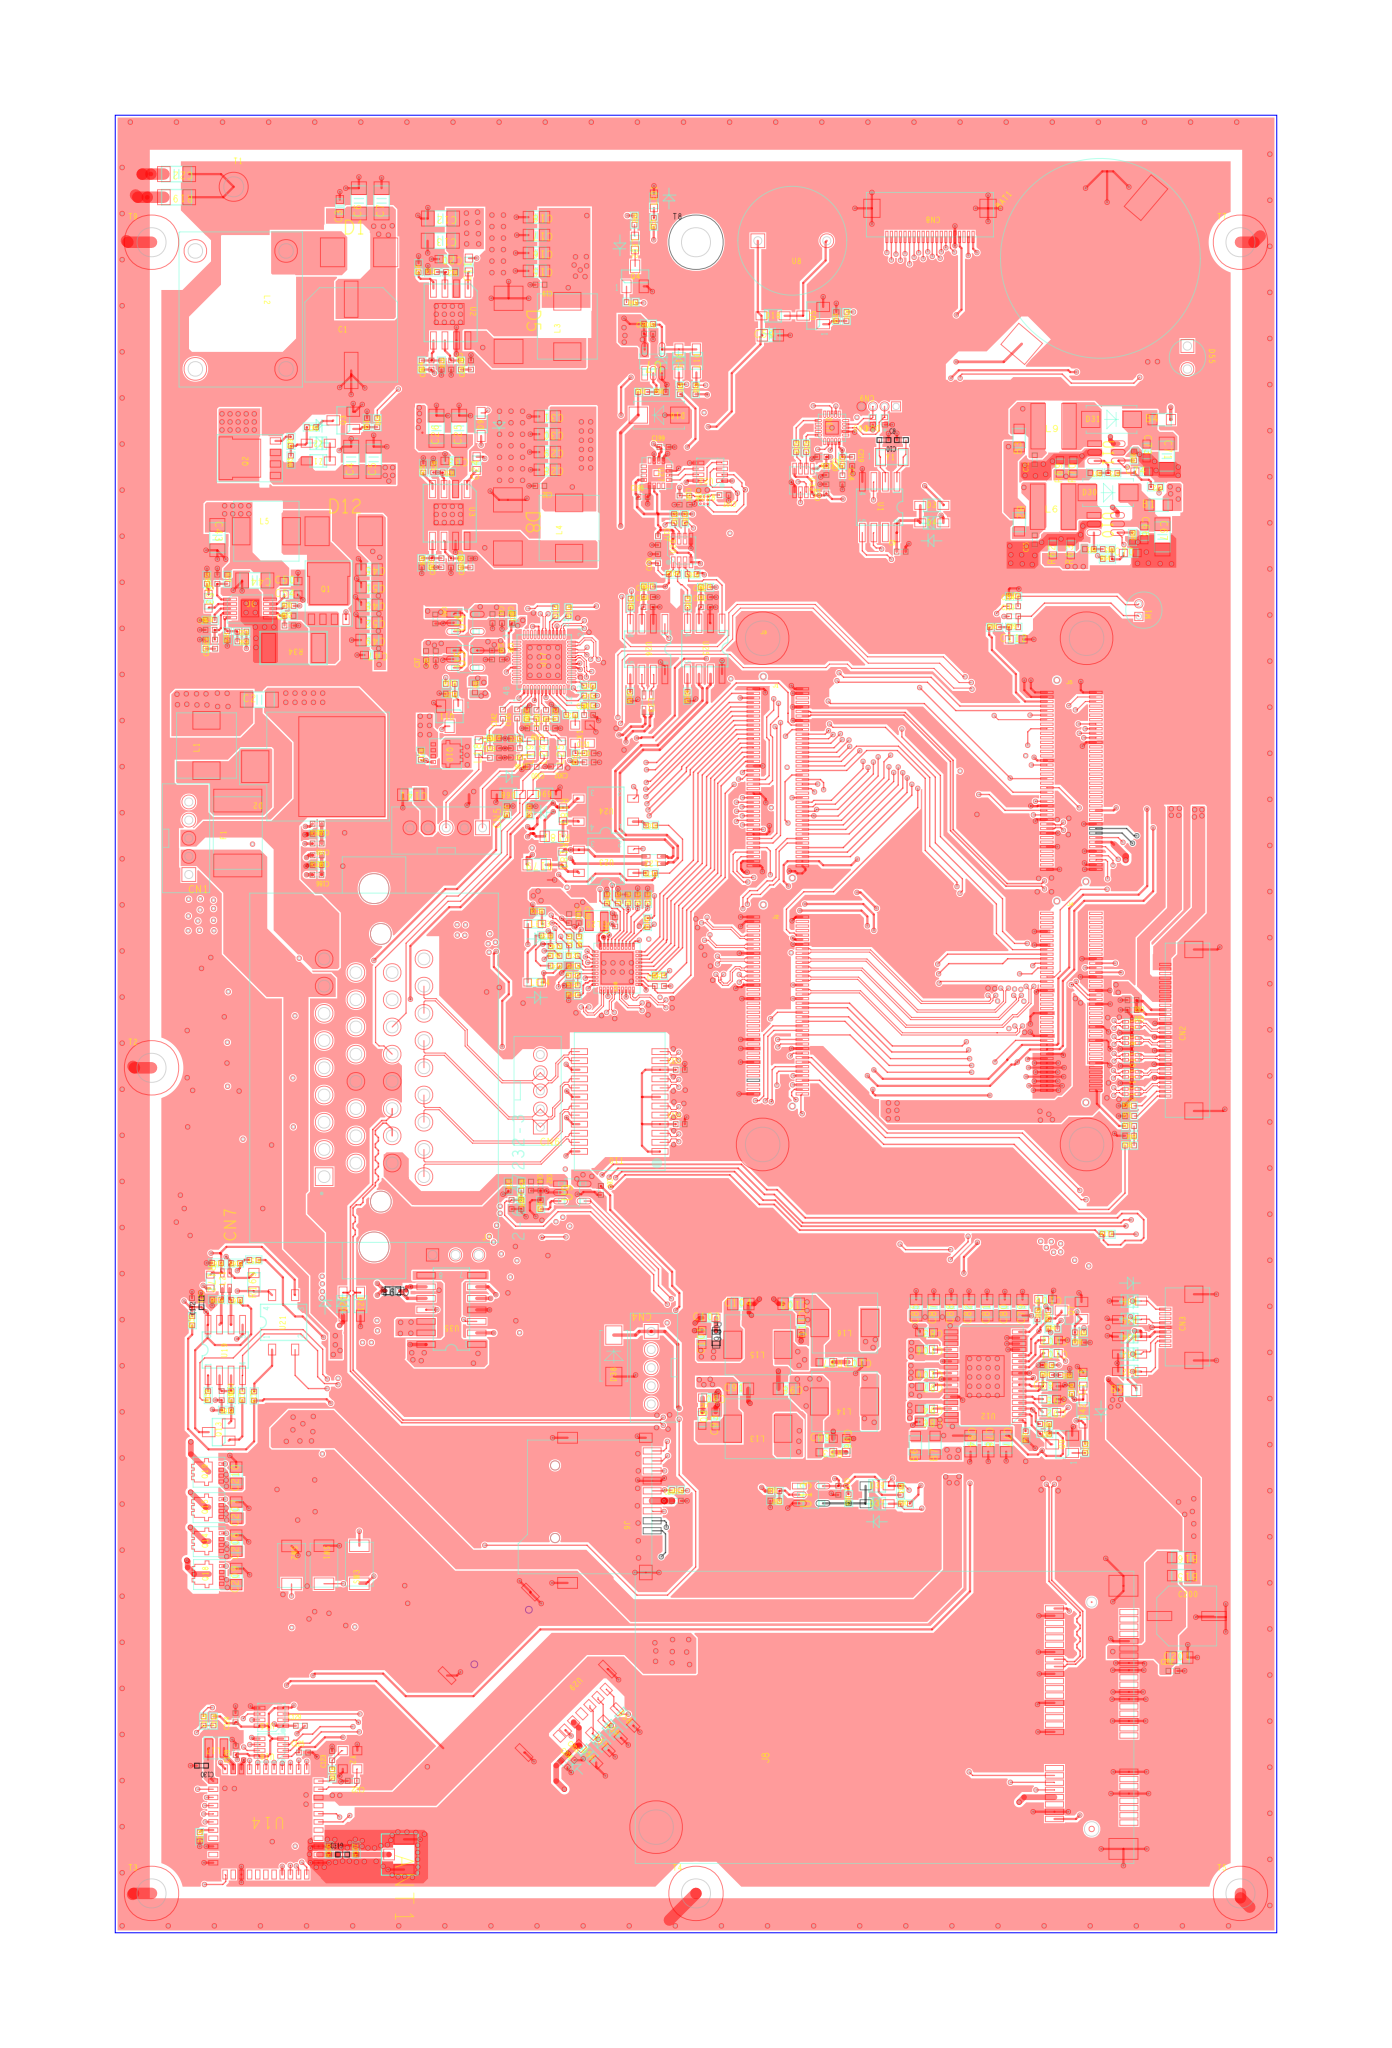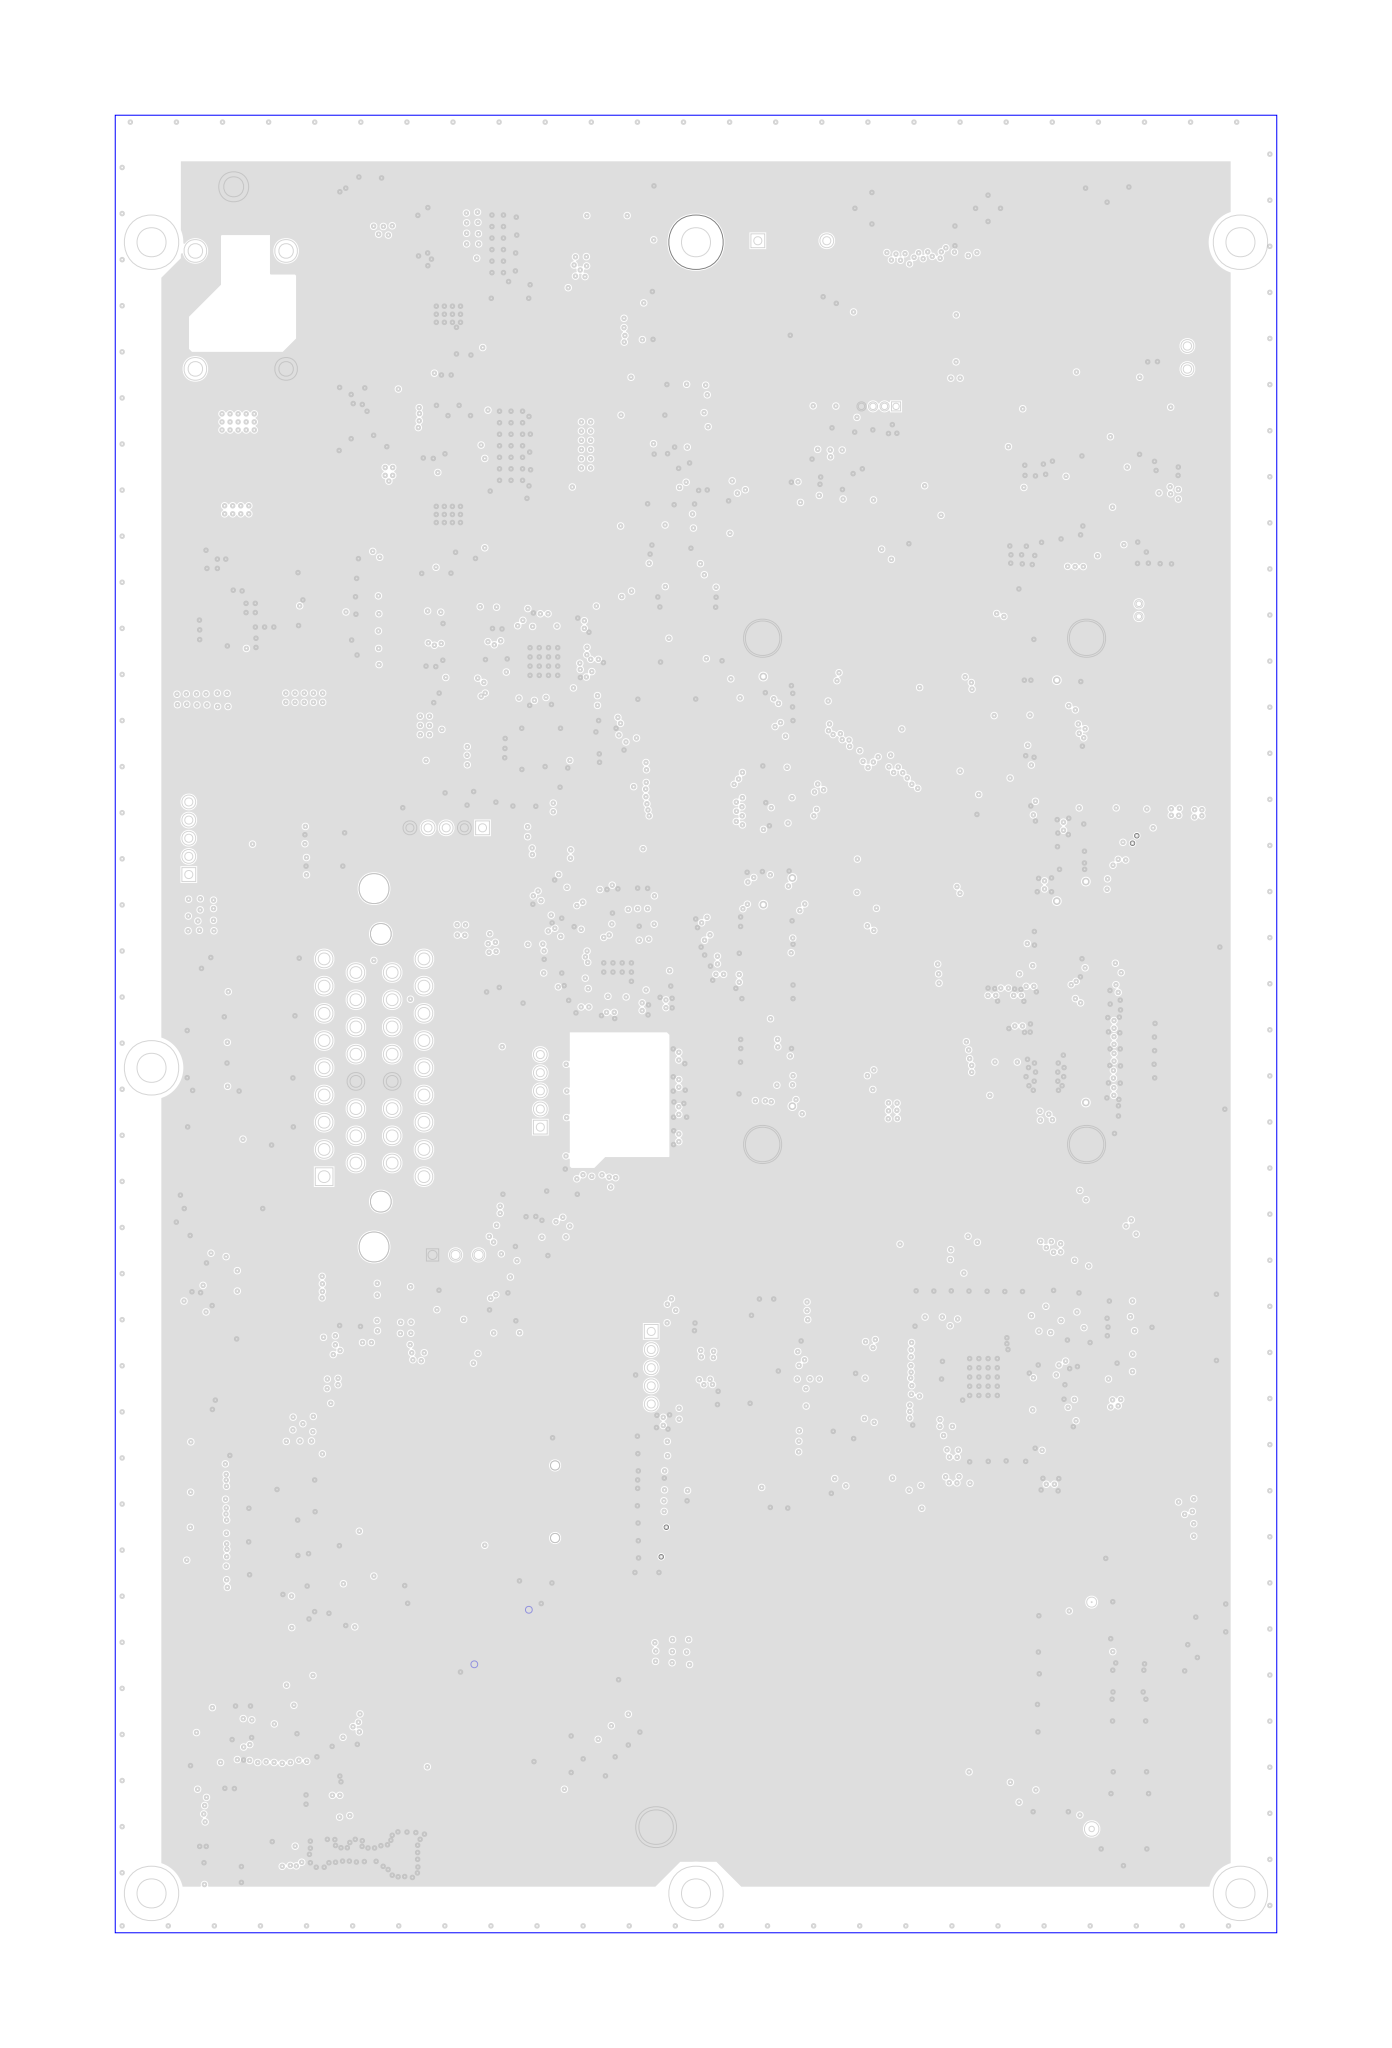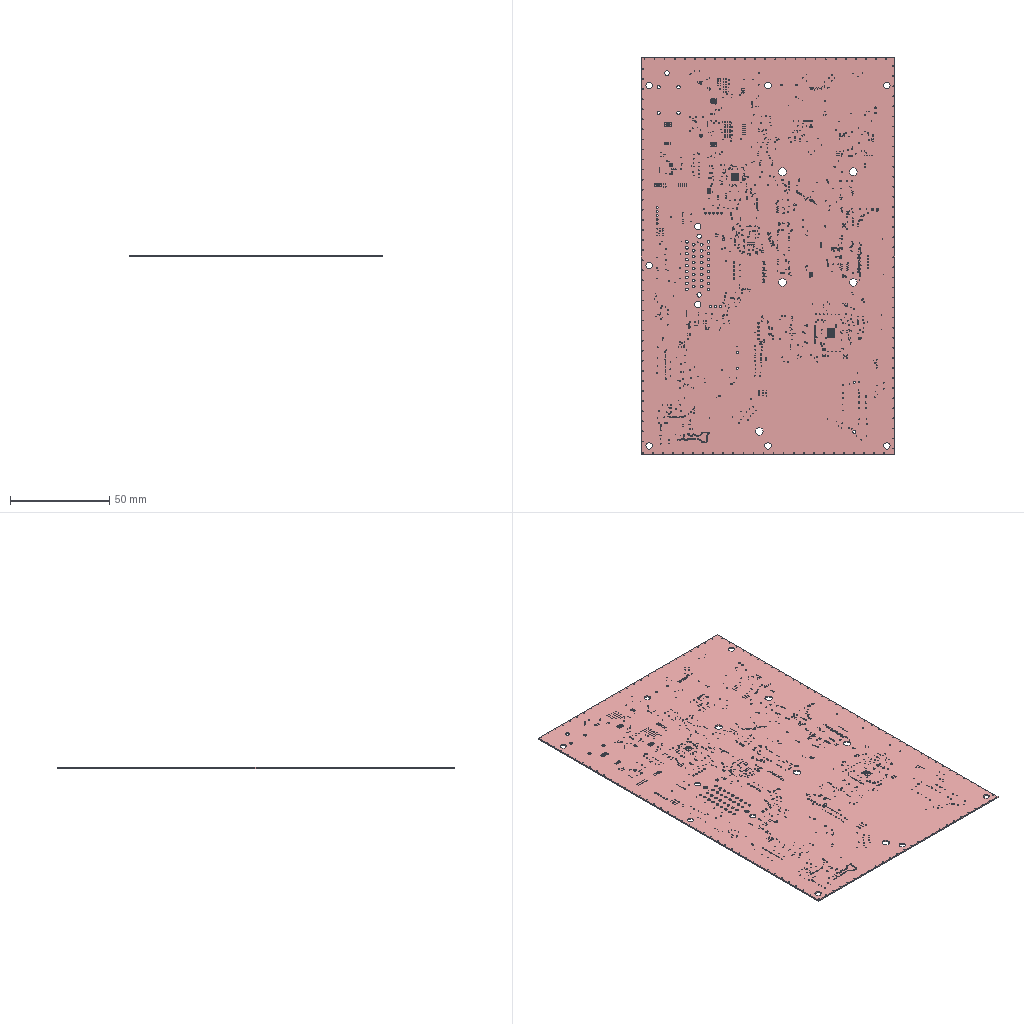Circuit board layout | Cadence Allegro | box 128 x 200.3 x 0.7 mm
Part placement, first 576 of 671 lines:
REFDES,COMP_VALUE,SYM_NAME,SYM_X,SYM_Y,SYM_ROTATE,SYM_MIRROR
ANT1,U.FL-R-SMT-1(80),IPEX,2427.527,1432.220,270.000,NO
B1,600R@100MHz,R0805,5701.296,7287.504,0.000,NO
B2,600R@100MHz,R0805,5097.120,7213.704,270.000,NO
B3,600R@100MHz,R0805,5096.136,7578.768,90.000,NO
B4,600R@100MHz,R0805,5715.072,7658.472,0.000,NO
B5,600R@100MHz,R0805,5564.520,3445.968,0.000,NO
B6,600R@100MHz,R0805,4645.948,3207.856,90.000,NO
B7,600R@100MHz,R0805,4731.556,3208.840,90.000,NO
B8,120R@100MHz,R0402,2865.408,6493.416,90.000,YES
B9,120R@100MHz,R0402,2735.520,6494.400,270.000,NO
B10,120R@100MHz,R0402,2896.896,6795.504,270.000,NO
B11,120R@100MHz,R0402,2835.888,6637.080,90.000,YES
B12,120R@100MHz,R0402,3170.448,6191.328,90.000,NO
B13,120R@100MHz,R0402,3366.264,5440.536,90.000,YES
B14,120R@100MHz,R0402,3001.200,5426.760,180.000,YES
B15,600R@100MHz,R0805,5799.696,2642.040,180.000,NO
B16,600R@100MHz,R0805,5799.680,2720.260,180.000,NO
BAT1,BS-08-B2AA008,CR2032,5433.821,8371.220,49.638,NO
C1,220uF,ED10,2198.256,8026.488,0.000,NO
C2,10uF,C1206,1799.736,6443.232,0.000,NO
C3,0.1uF,C0603,2149.056,8583.432,90.000,NO
C4,10uF,C1206,2198.256,7486.272,90.000,NO
C5,10uF,C1206,2295.672,7486.272,90.000,NO
C6,10uF,C1206,2231.712,8608.032,90.000,NO
C7,10uF,C1206,2330.112,8608.032,90.000,NO
C8,9pF,C0402,4585.440,7569.912,0.000,NO
C9,0.1uF,C0402,4584.456,7085.784,0.000,NO
C10,9pF,C0402,4509.672,7569.912,180.000,NO
C11,0.1uF,C0603,2708.952,8329.560,90.000,NO
C12,10uF,C1206,2585.952,8531.280,180.000,NO
C13,10uF,C1206,2584.968,8434.848,180.000,NO
C14,4.7nF,C0402,2546.592,7895.616,90.000,NO
C15,47uF,C0805,3002.184,8303.976,180.000,NO
C16,47uF,C0805,3002.184,8381.712,180.000,NO
C17,47uF,C0805,3002.184,8459.448,180.000,NO
C18,47uF,C0805,3002.184,8537.184,180.000,NO
C19,0.1uF,C0402,3017.928,8243.952,180.000,NO
C20,0.1uF,C0603,2609.568,8355.144,180.000,NO
C21,4.7nF,C0402,2632.200,7895.616,270.000,NO
C22,1nF,C1206,1440.576,8724.144,180.000,NO
C23,4.7nF,C0402,2717.808,7895.616,90.000,NO
C24,0.1uF,C0603,2742.408,7467.576,90.000,NO
C25,10uF,C1206,2666.640,7621.080,90.000,NO
C26,10uF,C1206,2568.240,7621.080,90.000,NO
C27,4.7nF,C0402,2589.888,7037.568,90.000,NO
C28,47uF,C0805,3049.416,7441.008,180.000,NO
C29,47uF,C0805,3049.416,7517.760,180.000,NO
C30,47uF,C0805,3049.416,7595.496,180.000,NO
C31,47uF,C0805,3049.416,7672.248,180.000,NO
C32,0.1uF,C0402,3016.944,7371.144,180.000,NO
C33,0.1uF,C0603,2635.152,7479.384,180.000,NO
C34,4.7nF,C0402,2631.216,7036.584,270.000,NO
C35,0.1uF,C0402,2565.288,6635.112,90.000,NO
C36,4.7nF,C0402,2715.840,7036.584,90.000,NO
C37,10uF,C0402,2522.976,6635.112,90.000,NO
C38,0.1uF,C0402,2852.616,6637.080,270.000,NO
C39,10uF,C0402,2809.320,6637.080,270.000,NO
C40,10uF,C0402,2563.320,6793.536,270.000,NO
C41,10uF,C0402,2811.288,6795.504,270.000,NO
C42,0.1uF,C0402,2852.616,6795.504,270.000,NO
C43,10uF,C1206,1617.696,7146.792,270.000,NO
C44,10uF,C1206,1780.056,6960.816,180.000,NO
C45,22uF,C0805,2275.992,7008.048,180.000,NO
C46,120pF,C0402,1617.696,6965.736,90.000,NO
C47,0.1uF,C0603,2285.832,6637.080,180.000,NO
C48,22uF,C0805,2275.992,6854.544,180.000,NO
C49,22uF,C0805,2275.992,6702.024,180.000,NO
C50,0.1uF,C0603,1937.496,6957.864,0.000,NO
C51,22uF,C0805,2275.992,6931.296,180.000,NO
C52,22uF,C0805,2275.992,6777.792,180.000,NO
C53,220nF,C0603,1579.320,6870.288,270.000,NO
C54,1uF,C0603,1937.496,6899.808,0.000,NO
C55,22nF,C0402,1607.856,6684.312,90.000,NO
C56,39pF,C0402,1586.208,6746.304,0.000,NO
C57,100pF,C0402,1928.640,6765.000,0.000,NO
C58,0.1uF,C0402,3488.280,8031.408,0.000,NO
C59,22uF,C0805,4016.688,8024.520,0.000,NO
C60,10uF,C0402,3281.640,4313.856,270.000,NO
C61,10uF,C0402,2978.568,4332.552,270.000,NO
C62,10uF,C0402,3019.896,4332.552,270.000,NO
C63,0.1uF,C0402,2893.944,4252.848,270.000,NO
C64,10uF,C0402,3609.312,2966.760,0.000,NO
C65,10uF,C0402,5164.032,7136.952,90.000,NO
C66,1uF,C0603,5639.304,7167.456,270.000,NO
C67,10uF,C1206,5718.024,7149.744,270.000,NO
C68,0.1uF,C0402,5586.168,5139.432,180.000,NO
C69,10uF,C0402,5586.168,5097.120,180.000,NO
C70,1uF,C0603,5578.296,7079.880,0.000,NO
C71,10uF,C1206,5736.720,7500.048,270.000,NO
C72,10uF,C0402,5164.032,7484.304,90.000,NO
C73,1uF,C0603,5649.144,7522.680,270.000,NO
C74,1uF,C0603,5628.480,7433.136,0.000,NO
C75,10uF,C0402,5577.312,3681.144,0.000,YES
C76,0.1uF,C0402,5577.312,3723.456,0.000,YES
C77,22uF,C0805,5040.048,3214.728,270.000,NO
C78,22uF,C0805,4962.312,3214.728,270.000,NO
C79,22uF,C0805,5110.896,3805.128,90.000,NO
C80,22uF,C0805,5034.144,3805.128,90.000,NO
C81,22uF,C0805,4957.392,3805.128,90.000,NO
C82,22uF,C0805,4878.672,3805.128,90.000,NO
C83,0.1uF,C0603,4694.664,3697.872,180.000,NO
C84,22uF,C0805,4885.560,3214.728,270.000,NO
C85,22uF,C0805,4649.400,3805.128,90.000,NO
C86,0.1uF,C0603,4693.680,3309.192,180.000,NO
C87,22uF,C0805,4726.152,3805.128,90.000,NO
C88,22uF,C0805,4801.920,3805.128,90.000,NO
C89,1uF,C0603,5228.976,3463.680,0.000,NO
C90,10nF,C0603,3752.976,3414.480,180.000,NO
C91,680nF,C0805,3886.800,3452.856,0.000,NO
C92,1uF,C0603,5228.976,3351.504,180.000,NO
C93,1nF,C0603,3779.544,3321.984,90.000,NO
C94,220nF,C0603,4694.664,3365.280,180.000,NO
C95,1uF,C0603,5228.976,3407.592,180.000,NO
C96,10nF,C0603,4346.328,3206.856,270.000,NO
C97,220nF,C0603,4694.664,3461.712,180.000,NO
C98,680nF,C0805,4086.552,3452.856,180.000,NO
C99,1nF,C0603,4259.736,3236.376,0.000,NO
C100,220nF,C0603,4694.664,3518.784,180.000,NO
C101,1uF,C0603,5235.864,3607.344,180.000,NO
C102,1uF,C0603,5236.848,3664.416,180.000,NO
C103,10nF,C0603,3751.008,3760.848,0.000,NO
C104,680nF,C0805,3888.768,3820.872,0.000,NO
C105,1nF,C0603,3721.488,3675.240,90.000,NO
C106,220nF,C0603,4694.664,3624.072,180.000,NO
C107,10nF,C0603,4385.688,3568.968,180.000,NO
C108,1uF,C0603,5211.264,3841.536,180.000,NO
C109,680nF,C0805,4107.216,3821.856,180.000,NO
C110,1nF,C0603,4150.512,3723.456,270.000,NO
C111,0.1uF,C0402,4311.888,3012.024,270.000,NO
C112,10uF,C0603,5083.344,6704.976,0.000,NO
C113,0.1uF,C0402,5072.520,6805.344,0.000,NO
C114,0.1uF,C0402,5072.520,6848.640,0.000,NO
C115,22uF,C0805,5124.672,3214.728,90.000,YES
C116,22uF,C0805,5040.048,3213.744,90.000,YES
C117,22uF,C0805,4962.312,3213.744,90.000,YES
C118,1uF,C0603,5374.608,3494.184,90.000,NO
C119,9pF,C0402,2160.864,1431.720,0.000,NO
C120,10uF,C0402,2048.688,1650.168,0.000,YES
C121,0.1uF,C0402,2048.688,1690.512,0.000,YES
C122,18pF,C0402,2203.176,1751.520,180.000,NO
C123,18pF,C0402,2115.600,1860.744,90.000,NO
C124,0.1uF,C0402,1696.416,2026.056,90.000,NO
C125,0.1uF,C0402,1991.616,1874.520,0.000,NO
C126,10uF,C0402,1691.496,1762.344,90.000,YES
C127,0.1uF,C0402,1650.168,1762.344,90.000,YES
C128,0.1uF,C0402,1697.400,1883.376,90.000,NO
C129,0.1uF,C0402,1977.840,1990.632,0.000,NO
C130,4.7uF,C0402,1548.816,1817.448,180.000,NO
C131,0.1uF,C0402,2907.720,6493.416,270.000,YES
C132,0.1uF,C0402,2949.048,6493.416,270.000,YES
C133,0.1uF,C0402,3043.512,6493.416,270.000,YES
C134,0.1uF,C0402,2996.280,6493.416,270.000,YES
C135,0.1uF,C0402,3090.744,6715.800,90.000,YES
C136,0.1uF,C0402,3146.832,6606.576,0.000,YES
C137,0.1uF,C0402,3146.832,6565.248,0.000,YES
C138,0.1uF,C0402,2929.368,6582.960,180.000,YES
C139,0.1uF,C0402,3011.040,6715.800,90.000,YES
C140,0.1uF,C0402,3228.504,6376.320,0.000,NO
C141,22uF,C0805,2457.048,6030.936,180.000,NO
C142,0.1uF,C0402,2856.552,6380.256,90.000,NO
C143,180pF,C0402,2820.144,6191.328,0.000,NO
C144,180pF,C0402,2820.144,6232.656,0.000,NO
C145,0.1uF,C0402,2918.544,6381.240,90.000,NO
C146,180pF,C0402,2910.672,6192.312,180.000,NO
C147,180pF,C0402,2910.672,6232.656,180.000,NO
C148,0.1uF,C0402,3002.184,6379.272,90.000,NO
C149,0.1uF,C0402,3043.512,6379.272,90.000,NO
C150,0.1uF,C0402,3230.472,6171.648,0.000,NO
C151,0.1uF,C0402,3230.472,6211.008,0.000,NO
C152,1nF,C1206,2885.088,5071.536,90.000,YES
C153,10uF,C0402,3626.040,4837.344,0.000,NO
C154,0.1uF,C0402,3626.040,4601.184,0.000,NO
C155,1nF,C1206,3035.640,5016.432,0.000,YES
C156,4.7uF,C0402,3409.560,5440.536,270.000,YES
C157,10uF,C0402,3366.264,5362.800,90.000,YES
C158,0.1uF,C0402,3324.936,5362.800,90.000,YES
C159,4.7uF,C0402,3185.208,5493.672,270.000,NO
C160,0.1uF,C0402,3143.880,5493.672,270.000,NO
C161,0.1uF,C0402,3422.352,5362.800,90.000,YES
C162,4.7uF,C0402,3343.632,5478.912,90.000,NO
C163,0.1uF,C0402,3435.144,5201.424,0.000,YES
C164,0.1uF,C0402,3266.880,5197.488,180.000,YES
C165,0.1uF,C0402,3535.512,5200.440,0.000,NO
C166,4.7uF,C0402,3242.280,5395.272,90.000,YES
C167,0.1uF,C0402,3283.608,5362.800,90.000,YES
C168,0.1uF,C0402,3324.936,5203.392,270.000,YES
C169,0.1uF,C0402,3376.104,5203.392,270.000,YES
C170,0.1uF,C0402,3266.880,5239.800,180.000,YES
C171,0.1uF,C0402,1507.488,3826.776,270.000,NO
C172,10uF,C0402,1548.816,3826.776,90.000,NO
C173,0.1uF,C0402,3704.760,7386.888,180.000,YES
C174,0.1uF,C0402,3793.320,7387.872,0.000,YES
C175,120pF,C0402,1636.392,3423.336,270.000,NO
C176,120pF,C0402,1794.816,4269.576,180.000,YES
C177,0.1uF,C0402,3529.608,7134.000,270.000,NO
C178,0.1uF,C0402,3529.608,7055.280,90.000,NO
C179,120pF,C0402,1797.768,4510.656,180.000,YES
C180,1uF,C0603,2768.976,4214.472,180.000,YES
C181,1uF,C0603,2769.960,4157.400,180.000,YES
C182,0.1uF,C0402,3735.264,6888.000,0.000,NO
C183,4.7uF,C0402,3735.264,6844.704,0.000,NO
C184,0.1uF,C0402,3486.312,6845.688,0.000,NO
C185,4.7uF,C0402,3487.296,6888.984,0.000,NO
C186,100pF(NC),C0402,2049.672,5683.584,180.000,NO
C187,100pF(NC),C0402,2050.656,5768.208,180.000,NO
C188,100pF(NC),C0402,2050.656,5819.376,180.000,NO
C189,100pF(NC),C0402,2050.656,5904.984,180.000,NO
C190,0.1uF,C0402,2194.320,2458.032,0.000,YES
C191,0.1uF,C0402,1960.128,2454.096,180.000,YES
C192,4.7uF,C0402,5654.064,7957.608,90.000,YES
C193,0.1uF,C0402,5695.392,7957.608,90.000,YES
C194,0.1uF,C0402,5737.704,7956.624,90.000,YES
C195,4.7uF,C0402,3623.088,7309.152,270.000,NO
C196,0.1uF,C0402,3665.400,7309.152,270.000,NO
C197,4.7uF,C0402,3815.952,7330.800,180.000,NO
C198,0.1uF,C0402,3464.664,7323.912,0.000,NO
C199,0.1uF,C0402,3555.192,7539.408,0.000,NO
C200,220uF,ED63,5823.312,2466.888,0.000,NO
C201,47uF,C0805,5792.808,2286.816,0.000,NO
C202,0.1uF,C0402,5763.288,2228.760,0.000,NO
C203,9pF,C0402,3152.881,1855.118,315.000,NO
C204,0.1uF,C0402,3122.689,1824.834,315.000,NO
C205,22uF,C0805,1682.640,5110.896,0.000,YES
C206,22uF,C0805,1699.368,2782.752,90.000,NO
C207,22uF,C0805,1699.368,2926.416,90.000,NO
C208,22uF,C0805,1694.448,4906.224,0.000,YES
C209,22uF,C0805,1699.368,2638.104,90.000,NO
C210,22uF,C0805,1699.368,3077.952,90.000,NO
C211,22uF,C0805,1697.400,4696.632,0.000,YES
C212,22uF,C0805,1682.640,5324.424,0.000,YES
C216,0.1uF,C0402,4329.600,7397.712,270.000,NO
C218,10uF,C0402,4240.056,7497.096,180.000,NO
C219,0.1uF,C0402,4371.912,7477.416,270.000,NO
C220,0.1uF,C0402,4259.736,7438.056,270.000,NO
C221,0.1uF,C0402,4259.736,7358.352,90.000,NO
C291,10uF,C1206,2841.792,3565.032,180.000,YES
C292,0.1uF,C0603,2866.392,3645.720,180.000,YES
C293,0.1uF,C0402,3066.144,4059.984,180.000,YES
C294,0.1uF,C0402,2895.912,4039.320,180.000,YES
C295,10uF,C1206,2324.208,3574.872,0.000,YES
C296,0.1uF,C0603,2348.808,3653.592,0.000,YES
C297,1nF,C0603,2086.080,3987.168,0.000,YES
C298,1nF,C0603,2379.312,3877.944,180.000,NO
C299,180pF,C0402,2982.504,6319.248,180.000,NO
C300,180pF,C0402,2983.488,6151.968,180.000,NO
C301,180pF,C0402,3063.192,6319.248,0.000,NO
C302,180pF,C0402,3084.840,6152.952,180.000,NO
CN1,A2008WV-5P,A2008WV_5P,1493.712,5842.008,0.000,NO
CN2,X05A20H30G,FPC-30-0P5-2MMH,5730.315,5008.858,90.000,NO
CN3,KH-FG0.5-H2.0-9PIN,FPC-9-0P5-2MMH,5730.315,3719.488,90.000,NO
CN4,A2008WV-5P,A2008WV_5P,3500.088,3544.368,180.000,NO
CN5,A2008WV-5P,A2008WV_5P,2610.552,5887.272,90.000,NO
CN6,A2008WV-5P,A2008WV_5P,3018.912,4745.832,0.000,NO
CN7,TE_2_6447232_3,TE_2-6447232-3,2297.460,4845.927,90.000,NO
CN8,X05A20H20G,FPC-20-0P5-2MMH,4709.424,8451.576,180.000,NO
CN9,1.27-4P(NC),SIP4_1P27,4487.237,7716.135,180.000,NO
D1,MBRS360T3G,SMC,2232.696,8384.664,0.000,NO
D2,SM8S33A,DO_218AB,1969.968,6152.952,180.000,NO
D3,B5819WS,SOD323,4717.296,7286.520,270.000,NO
D4,B5819WS,SOD323,4717.296,7210.752,270.000,NO
D5,MBRS360T3G,SMC,2881.152,8069.784,270.000,NO
D8,MBRS360T3G,SMC,2878.200,7195.008,270.000,NO
D9,B5819WS,SOD323,2762.088,7637.808,0.000,NO
D11,JEB03CX,SOD323,5061.696,6158.856,90.000,YES
D12,MBRS360T3G,SMC,2165.784,7174.344,0.000,NO
D13,JEB03CX,SOD323,2332.080,2521.992,270.000,YES
D14,JEB03CX,SOD323,2331.096,2598.744,270.000,YES
D15,B5819WS,SOD323,3620.136,7913.328,180.000,NO
D16,SMAJ12A,SMA,3624.072,7678.152,180.000,NO
D17,B5819WS,SOD323,3695.904,7913.328,180.000,NO
D18,B5819WS,SOD323,4028.496,8109.144,270.000,NO
D19,0402ESDA-05N,R0402,2880.168,4332.552,270.000,NO
D20,JEB03CX,SOD323,2162.832,3820.872,180.000,NO
D21,JEB03CX,SOD323,2238.600,3819.888,180.000,NO
D22,JEB03CX,SOD323,3457.776,2945.112,90.000,YES
D23,JEB03CX,SOD323,3457.776,3096.648,90.000,YES
D24,JEB03CX,SOD323,3457.776,3171.432,90.000,YES
D25,JEB03CX,SOD323,3458.760,2718.792,90.000,YES
D26,JEB03CX,SOD323,3458.760,2793.576,90.000,YES
D27,JEB03CX,SOD323,3457.776,3020.880,90.000,YES
D28,JEB03CX,SOD323,3458.760,2870.328,90.000,YES
D29,JEB03CX,SOD323,3457.776,3247.200,90.000,YES
D30,SS34,SMA,5392.320,7341.624,0.000,NO
D31,SS34,SMA,5407.080,7659.456,0.000,NO
D32,JEB03CX,SOD323,5575.344,3527.640,90.000,NO
D33,JEB03CX,SOD323,5575.344,3603.408,90.000,NO
D34,JEB03CX,SOD323,5575.344,3679.176,90.000,NO
D35,JEB03CX,SOD323,5575.344,3752.976,90.000,NO
D36,JEB03CX,SOD323,5575.344,3833.664,90.000,NO
D37,B5819WS,SOD323,4480.152,2953.968,270.000,NO
D38,SMAJ12A,SMA,3337.728,3505.992,90.000,NO
D39,B5819WS,SOD323,4480.152,3031.704,270.000,NO
D40,B5819WS,SOD323,5316.552,3822.840,270.000,YES
D41,B5819WS,SOD323,4767.480,3250.152,90.000,YES
D42,B5819WS,SOD323,5373.624,3356.424,0.000,NO
D43,B5819WS,SOD323,5258.496,3329.856,90.000,YES
D44,JEB03CX,SOD323,2644.992,6015.192,0.000,YES
D45,JEB03CX,SOD323,2767.992,6015.192,0.000,YES
D46,SMAJ7.0A,SMA,1520.280,4293.192,270.000,YES
D47,JEB03CX,SOD323,2710.920,3893.688,180.000,YES
D48,JEB03CX,SOD323,2578.080,3892.704,180.000,YES
D49,SMAJ7.0CA,SMA,1655.088,4293.192,270.000,YES
D50,SMAJ7.0A,SMA,1499.616,4176.096,180.000,YES
D51,PESD2CAN,SOT-23,2082.144,5720.976,270.000,YES
D52,PESD2CAN,SOT-23,2083.128,5855.784,270.000,YES
D53,JEB03CX,SOD323,2164.800,2521.992,270.000,YES
D54,JEB03CX,SOD323,1989.648,2520.024,90.000,YES
D55,HLPT550B3 H4,LED_D3MM,5826.264,7928.088,270.000,NO
D56,JEB03CX,SOD323,3225.939,1866.946,225.000,NO
D57,JEB03CX,SOD323,3279.515,1920.522,225.000,NO
D58,JEB03CX,SOD323,3386.667,2026.283,225.000,NO
D59,JEB03CX,SOD323,3332.395,1973.402,225.000,NO
D60,SMAJ12A,SMA,1547.832,5007.576,180.000,YES
D61,SMAJ12A,SMA,1549.800,4802.904,180.000,YES
D62,SMAJ12A,SMA,1548.816,4589.376,180.000,YES
D63,SMAJ12A,SMA,1548.816,5219.136,180.000,YES
D64,TPESD8L3.3CT5G,DFN1006_2L,4513.608,7652.568,180.000,NO
D65,TPESD8L3.3CT5G,DFN1006_2L,4461.456,7652.568,180.000,NO
D66,MURS260,SMA,1936.512,4164.288,180.000,YES
D67,MURS260,SMA,2211.048,3901.560,180.000,YES
D68,JEB03CX,SOD323,2880.168,6031.920,90.000,NO
D69,JEB03CX,SOD323,3036.624,6031.920,270.000,NO
F1,SMD2920P185TS,R2920,1706.256,5864.640,90.000,NO
F2,MF-NSMF012-2,R1206,1831.224,4341.408,180.000,YES
F3,MF-NSMF012-2,R1206,1831.224,4437.840,180.000,YES
F4,BSMD0603-001-60V,R0603,2280.912,5758.352,0.000,YES
F5,BSMD0603-001-60V,R0603,2280.912,5815.424,0.000,YES
F6,BSMD0603-001-60V,R0603,2280.912,5872.496,0.000,YES
F7,BSMD0603-001-60V,R0603,2280.912,5930.552,0.000,YES
F8,BSMD0603-001-60V,R0603,1854.840,4879.656,180.000,YES
F9,BSMD0603-001-60V,R0603,1854.840,4995.768,180.000,YES
F10,BSMD0603-001-60V,R0603,1852.872,4672.032,180.000,YES
F11,BSMD0603-001-60V,R0603,1854.840,5206.344,180.000,YES
J1,AXK5F80337YG,AXK5F80337YG,4049.266,6106.636,0.000,NO
J2,AXK5F80337YG,AXK5F80337YG,4049.266,5116.478,0.000,NO
J3,CON10,DIP-CORE-A40I,4684.109,5611.557,0.000,NO
J4,AXK5F80337YG,AXK5F80337YG,5322.888,5132.226,0.000,NO
J5,AXK5F80337YG,AXK5F80337YG,5322.888,6090.888,0.000,NO
J6,TF-012,TFCARD1,3082.872,3120.264,270.000,NO
J7,2.54-3P,SIP2P54_3,2651.249,4033.858,0.000,NO
J8,PCIE-52P40H,MINI-PCIE-SMD,5411.016,2027.040,90.000,NO
L1,10uH,IND0630,1570.464,6244.464,90.000,NO
L2,5mH,SQ1212WS,1719.048,8134.728,270.000,NO
L3,10uH,IND0630,3136.008,8062.896,90.000,NO
L4,10uH,IND0630,3143.880,7188.120,90.000,NO
L5,10uH,IND0630,1830.240,7174.344,0.000,NO
L6,47uH,IND5X5,5243.736,7280.616,0.000,NO
L7,ICMEF112P900MFR,ICMEF112P900MFR,5585.184,5034.144,270.000,NO
L8,ICMEF112P900MFR,ICMEF112P900MFR,5585.184,4964.280,270.000,NO
L9,47uH,IND5X5,5245.704,7629.936,0.000,NO
L10,ICMEF112P900MFR,ICMEF112P900MFR,5585.184,4891.464,270.000,NO
L11,ICMEF112P900MFR,ICMEF112P900MFR,5585.184,4817.664,270.000,NO
L12,ICMEF112P900MFR,ICMEF112P900MFR,5584.200,4742.880,270.000,NO
L13,10uH,IND0630,3962.568,3279.672,180.000,NO
L14,10uH,IND0630,4338.456,3397.752,180.000,NO
L15,10uH,IND0630,3962.568,3643.752,180.000,NO
L16,10uH,IND0630,4340.424,3738.216,180.000,NO
L17,2.2uH,L2520,1613.760,1894.200,180.000,NO
L18,1.8uH,R0603,2752.248,6237.576,90.000,NO
L19,1.8uH,R0603,2978.568,6232.656,90.000,NO
L20,2.2uH,L2520,3263.928,5480.880,180.000,NO
L21,90R,WCM2012,1655.088,3922.224,90.000,NO
L22,90R,WCM2012,3510.912,5747.544,180.000,NO
L23,90R,WCM2012,3484.344,6430.440,270.000,NO
L24,1.8uH,R0603,3035.640,6233.640,90.000,NO
L25,1.8uH,R0603,3111.408,6232.656,90.000,NO
LED1,RED,D0603,3511.896,8608.032,90.000,NO
LED2,GREEN,LED_0603,3429.240,8425.008,270.000,NO
LED3,YELLOW,D0603,2995.296,5470.056,0.000,NO
LED4,GREEN,D0603,2994.312,5216.184,0.000,NO
M1,GMI4015P-2C-32db,MIC4015P,5637.336,6831.912,90.000,NO
Q1,HSBA20N15S,DFN5X6,2100.840,6947.040,0.000,NO
Q2,HSBA0139,DFN5X6,1715.112,7491.192,90.000,NO
Q3,2N7002KQ-7,SOT-23,2163.816,7655.520,90.000,NO
Q4,MMBT3904,SOT-23,3430.224,8280.360,0.000,NO
Q5,SS8050,SOT-23,4202.664,8110.128,90.000,NO
Q6,MMBT3904,SOT-23,4975.104,5941.392,270.000,YES
Q7,SS8050,SOT-23,5323.440,3792.336,90.000,NO
Q8,SS8550,SOT-23,5312.616,3220.632,270.000,YES
Q9,SS8050,SOT-23,5283.096,3211.776,90.000,NO
Q10,AON7407,DFN3X3,2609.568,6211.008,270.000,NO
Q11,MMBT3904,SOT-23,2625.312,6371.400,180.000,NO
Q12,2N7002KQ-7,SOT-23,2831.952,3943.872,90.000,YES
Q13,MMBT3904,SOT-23,1623.600,3264.912,90.000,NO
Q14,HSBB2627,DFN3X3,1580.304,2787.672,90.000,NO
Q15,HSBB2627,DFN3X3,1579.320,2935.272,90.000,NO
Q16,SS8050,SOT-23,1875.504,2920.512,90.000,YES
Q17,SS8050,SOT-23,1874.520,2775.864,90.000,YES
Q18,HSBB2627,DFN3X3,1581.288,2644.992,90.000,NO
Q19,HSBB2627,DFN3X3,1579.320,3088.776,90.000,NO
Q20,SS8050,SOT-23,1874.520,2634.168,90.000,YES
Q21,SS8050,SOT-23,1875.504,3065.160,90.000,YES
R1,2.2K,R0402,4290.240,5958.120,0.000,YES
R2,2.2K,R0402,4289.256,5902.032,0.000,YES
R3,2.2K,R0402,4019.640,6111.608,0.000,YES
R4,2.2K,R0402,4019.640,6054.536,0.000,YES
R5,0R,R0402,4033.416,5407.080,180.000,YES
R6,0R(NC),R0402,5596.008,5974.848,0.000,YES
R7,0R,R0402,4074.744,5603.880,180.000,YES
R8,0R,R0402,5060.712,4924.920,0.000,YES
R9,0R(NC),R0402,4033.416,5464.152,180.000,YES
R10,0R,R0402,5596.008,5916.792,0.000,YES
R11,0R(NC),R0402,4074.744,5546.808,180.000,YES
R12,1M,R0402,2629.248,8299.056,180.000,NO
R13,100K,R0402,2550.528,8299.056,0.000,NO
R14,53.6K,R0402,2504.280,7895.616,90.000,NO
R15,10K,R0402,5111.880,5288.016,180.000,YES
R16,200K,R0402,2490.504,8317.752,90.000,NO
R17,20K,R0402,2674.512,7895.616,270.000,NO
R18,10.2K,R0402,2589.888,7895.616,270.000,NO
R19,1M,R1206,1440.576,8623.776,180.000,NO
R20,1M(NC),R0402,2615.472,7429.200,180.000,NO
R21,100K,R0402,2554.464,7448.880,270.000,NO
R22,43K,R0402,2547.576,7037.568,90.000,NO
R23,10.2K,R0402,3510.912,8514.552,90.000,NO
R24,20K,R0402,2673.528,7036.584,270.000,NO
R25,200K,R0402,2511.168,7448.880,90.000,NO
R26,10.2K,R0402,2504.280,7037.568,270.000,NO
R27,220K,R0402,1660.992,6965.736,270.000,NO
R28,10K,R0402,1572.432,6965.736,270.000,NO
R29,100K,R0402,1586.208,6788.616,0.000,NO
R30,10R,R0402,1928.640,6850.608,0.000,NO
R31,20K,R0402,1566.528,6684.312,270.000,NO
R32,1K,R0402,1928.640,6807.312,0.000,NO
R33,2.2K,R0402,1660.992,6720.720,90.000,NO
R34,0.01R,R2512,1948.320,6667.584,180.000,NO
R35,75K,R0402,1723.968,6738.432,180.000,NO
R36,75K,R0402,1723.968,6696.120,180.000,NO
R37,10K,R0402,5575.344,4593.312,0.000,NO
R38,1K,R0402,5575.344,4508.688,0.000,NO
R39,22R,R0402,1936.512,7564.008,90.000,NO
R40,10K,R0402,3488.280,8073.720,180.000,NO
R41,10K,R0402,3624.072,7788.360,270.000,NO
R42,1K,R0402,3427.272,8524.392,270.000,NO
R43,100K,R0402,3462.696,7778.520,0.000,NO
R44,100K,R0402,5575.344,4551.000,180.000,NO
R45,10K,R0402,1936.512,7482.336,90.000,NO
R46,31.6K,R0402,3543.384,7778.520,0.000,NO
R47,4.7K,R0402,2026.056,7626.000,180.000,NO
R48,10K,R0402,3691.968,7788.360,270.000,NO
R49,1K,R0402,3412.512,8168.184,180.000,NO
R50,10K,R0402,2311.416,7645.680,270.000,NO
R51,100K,R0402,2267.136,7645.680,90.000,NO
R52,10K,R0402,4347.312,8106.192,270.000,NO
R53,100K,R0402,4303.032,8106.192,90.000,NO
R54,20K,R0402,2936.256,4332.552,270.000,NO
R55,4.7K,R0402,3019.896,4251.864,90.000,NO
R56,20K,R0402,2936.256,4252.848,270.000,NO
R57,100R,R0402,5102.040,5941.392,0.000,YES
R58,1K,R0402,4865.880,5929.584,90.000,YES
R59,22R,R0402,3610.296,3013.008,180.000,NO
R60,100K,R0402,5588.136,7147.776,270.000,NO
R61,10K,R0402,5401.176,7096.608,180.000,NO
R62,3.3R,R0603,5242.752,7099.560,90.000,NO
R63,3.3R,R0603,5320.488,7099.560,90.000,NO
R64,75K,R0402,5478.912,7054.296,0.000,NO
R65,2.49K,R0402,5478.912,7096.608,180.000,NO
R66,100K,R0402,5595.024,7501.032,90.000,NO
R67,10K,R0402,5424.792,7427.232,180.000,NO
R68,10K,R0402,5574.360,4680.888,0.000,NO
R69,10R,R0603,5273.256,7453.800,90.000,NO
R70,10R(NC),R0603,5331.328,7453.800,90.000,NO
R71,10K,R0402,5575.344,4636.608,0.000,NO
R72,75K,R0402,5688.504,7366.224,180.000,NO
R73,2.49K,R0402,5502.528,7427.232,180.000,NO
R74,22R,R0402,5538.936,3835.632,180.000,YES
R75,22R,R0402,5539.920,3767.736,180.000,YES
R76,22R,R0402,5538.936,3605.376,180.000,YES
R77,22R,R0402,5539.920,3527.640,180.000,YES
R78,0R,R0402,5217.168,3556.176,180.000,NO
R79,1K,R0402,5124.672,3249.168,90.000,NO
R80,3.3R,R0603,3721.488,3321.984,270.000,NO
R81,100K,R0402,5207.328,3300.336,180.000,NO
R82,100K,R0402,5207.328,3258.024,180.000,NO
R83,3.3R,R0603,4259.736,3177.336,180.000,NO
R84,100K,R0402,5218.152,3512.880,0.000,NO
R85,20K,R0402,5295.888,3512.880,180.000,NO
R86,3.3R,R0603,3781.512,3674.256,270.000,NO
R87,3.3R,R0603,4259.736,3567.984,180.000,NO
R88,4.7K,R0402,5175.840,3773.640,270.000,NO
R89,10K,R0402,4356.168,2975.616,90.000,NO
R90,10K,R0402,4602.168,2953.968,0.000,NO
R91,100K,R0402,4036.368,3009.072,0.000,NO
R92,31.6K,R0402,4036.368,2966.760,180.000,NO
R93,10K,R0402,4582.488,3012.024,270.000,NO
R94,240R,R0402,5242.752,3713.616,0.000,NO
R95,100K,R0402,5223.072,3773.640,90.000,NO
R96,100R,R0402,4988.880,6758.112,0.000,NO
R97,10K,R0402,5357.880,3697.872,180.000,NO
R98,100K,R0402,5357.880,3653.592,0.000,NO
R99,1K,R0402,5072.520,6758.112,0.000,NO
R100,1K,R0402,4879.656,3250.152,180.000,YES
R101,100K,R0402,5188.632,3235.392,90.000,YES
R102,10K,R0402,5202.408,3167.496,180.000,YES
R103,1K,R0402,5071.536,6891.936,0.000,NO
R104,10K,R0402,5325.408,3449.904,90.000,NO
R105,1M,R0402,5382.480,3194.064,270.000,NO
R106,0R(NC),R0402,2101.824,1451.400,90.000,NO
R107,0R(NC),R0402,2219.904,1451.400,90.000,NO
R108,22R,R0402,2115.600,1782.024,270.000,NO
R109,0R,R0402,1899.120,1436.640,270.000,YES
R110,10K(NC),R0402,1855.824,1436.640,270.000,YES
R111,0R(NC),R0402,1540.944,1509.456,270.000,NO
R112,10K,R0402,1600.968,2011.296,270.000,NO
R113,22R,R0402,1557.672,2011.296,270.000,NO
R114,22R,R0402,3140.928,6825.024,270.000,NO
R115,22R,R0402,3083.856,6825.024,270.000,NO
R116,22R,R0402,3228.504,6418.632,180.000,NO
R117,10K,R0402,2500.344,6202.152,270.000,NO
R118,10K,R0402,2628.264,6512.112,0.000,NO
R119,75R,R0402,2820.144,6275.952,0.000,NO
R120,20K,R0402,2628.264,6468.816,180.000,NO
R121,75R,R0402,2910.672,6274.968,180.000,NO
R122,75R,R0402,2959.872,6379.272,90.000,NO
R123,75R,R0402,3085.824,6379.272,90.000,NO
R124,4.7K(NC),R0402,3228.504,6460.944,180.000,NO
R125,4.7K(NC),R0402,3228.504,6504.240,180.000,NO
R126,22R,R0402,3150.768,6377.304,180.000,NO
R127,0R,R0402,2673.528,5319.504,180.000,YES
R128,1M,R1206,2785.704,5071.536,90.000,YES
R129,0R,R0402,3161.592,5289.000,180.000,NO
R130,120R,R0402,3161.592,5203.392,0.000,NO
R131,75R,R0402,3111.408,4483.104,0.000,YES
R132,75R,R0402,3111.408,4601.184,0.000,YES
R133,100R,R0402,3161.592,5245.704,0.000,NO
R134,75R,R0402,3111.408,4719.264,0.000,YES
R135,100R,R0402,3161.592,5331.312,0.000,NO
R136,75R,R0402,3111.408,4838.328,0.000,YES
R137,120R,R0402,3143.880,5396.256,270.000,NO
R138,1K,R0402,3006.120,5523.192,0.000,NO
R139,1K,R0402,3043.512,5419.872,180.000,NO
R140,4.7K,R0402,3082.872,5374.608,180.000,NO
R141,4.7K,R0402,3082.872,5289.000,180.000,NO
R142,4.7K,R0402,3082.872,5331.312,0.000,NO
R143,2.49K,R0402,3161.592,5161.080,0.000,NO
R144,10K,R0402,3186.192,5396.256,270.000,NO
R145,4.7K,R0402,3483.360,5475.960,90.000,NO
R146,4.7K,R0402,3308.208,5578.296,270.000,NO
R147,4.7K,R0402,3355.440,5578.296,270.000,NO
R148,4.7K,R0402,3398.736,5578.296,270.000,NO
R149,4.7K(NC),R0402,3398.736,5578.296,270.000,YES
R150,4.7K,R0402,3441.048,5578.296,270.000,NO
R151,4.7K(NC),R0402,3441.048,5578.296,270.000,YES
R152,4.7K(NC),R0402,3484.344,5578.296,270.000,NO
R153,4.7K,R0402,3484.344,5578.296,270.000,YES
R154,1.8K,R0402,3535.512,5246.688,0.000,NO
R155,0R,R0402,1508.472,3748.056,90.000,NO
R156,100R,R0402,2638.104,3924.192,270.000,YES
R157,0R(NC),R0402,1776.120,4011.768,180.000,NO
R158,1K(NC),R0402,1614.744,3839.568,180.000,NO
R159,240R,R0402,1577.352,3423.336,90.000,NO
R160,1K(NC),R0402,1614.744,3998.976,180.000,NO
R161,240R,R0402,1678.704,3423.336,90.000,NO
R162,10K(NC),R0402,3599.472,7229.448,270.000,NO
R163,10K(NC),R0402,3644.736,7229.448,270.000,NO
R164,10K(NC),R0402,3595.536,6988.368,0.000,NO
R165,10K(NC),R0402,3677.208,6988.368,180.000,NO
R166,4.7K,R0402,1658.040,3359.376,180.000,NO
R167,1K(NC),R0402,1696.416,3838.584,180.000,NO
R168,1K(NC),R0402,1696.416,3997.992,180.000,NO
R169,120R,R0805,1776.120,3915.336,90.000,NO
R170,470R,R0402,1777.104,3421.368,90.000,NO
R171,1K,R0402,1725.936,3423.336,90.000,NO
R172,0R(NC),R0603,1587.192,3918.288,270.000,NO
R173,0R,R0402,5476.944,4123.944,0.000,NO
R174,0R,R0402,3735.264,6931.296,0.000,NO
R175,0R,R0402,3487.296,6934.248,0.000,NO
R176,0R,R0402,2050.656,5725.896,0.000,NO
R177,0R,R0402,2050.656,5861.688,0.000,NO
R178,470R,R0402,3496.152,5690.472,180.000,NO
R179,120R,R0805,3003.168,5726.880,180.000,NO
R180,0R(NC),R0603,3115.344,5753.448,270.000,NO
R181,120R,R0805,3077.936,5850.364,180.000,NO
R182,470R,R0402,3497.136,5898.096,180.000,NO
R183,0R(NC),R0603,3117.312,5946.312,270.000,NO
Pad and via stacks, first 104 of 320 lines:
# Allegro (Cadence) via spans and padstacks; design units: ("mils" 3 1000)
# via spans: padstack,start_layer,end_layer,net_example,count
0503,ETCH/TOP,ETCH/BOTTOM,EGND,1695
# Allegro padstack definitions: name,start_layer,end_layer,drill,plating,holeType,type
PAD3,"ETCH/TOP","ETCH/TOP",0.0,"NON_PLATED","none","smd"
PAD2,"ETCH/TOP","ETCH/TOP",0.0,"NON_PLATED","none","smd"
PAD4,"ETCH/TOP","ETCH/TOP",0.0,"NON_PLATED","none","smd"
PAD1,"ETCH/TOP","ETCH/TOP",0.0,"NON_PLATED","none","smd"
PAD5,"ETCH/TOP","ETCH/TOP",0.0,"NON_PLATED","none","smd"
03502,"ETCH/TOP","ETCH/BOTTOM",7.87,"PLATED","circle_drill","through"
0503,"ETCH/TOP","ETCH/BOTTOM",11.811,"PLATED","circle_drill","through"
R028X033S,"ETCH/TOP","ETCH/TOP",0.0,"PLATED","none","smd"
R018X020S,"ETCH/TOP","ETCH/TOP",0.0,"PLATED","none","smd"
CAP-8X9-DIP,"ETCH/TOP","ETCH/BOTTOM",23.622,"PLATED","circle_drill","through"
C0805,"ETCH/TOP","ETCH/TOP",0.0,"PLATED","none","smd"
CASE-B,"ETCH/TOP","ETCH/TOP",0.0,"NON_PLATED","none","smd"
DO-214AC,"ETCH/TOP","ETCH/TOP",0.0,"NON_PLATED","none","smd"
SOD-323,"ETCH/TOP","ETCH/TOP",0.0,"NON_PLATED","none","smd"
PAD49,"ETCH/TOP","ETCH/TOP",0.0,"NON_PLATED","none","smd"
L0603,"ETCH/TOP","ETCH/TOP",0.0,"NON_PLATED","none","smd"
DC044A,"ETCH/TOP","ETCH/BOTTOM",31.496,"PLATED","oval slot","through"
DC044A-1,"ETCH/TOP","ETCH/BOTTOM",86.614,"NON_PLATED","circle_drill","through"
FPC30P-0D5-11,"ETCH/TOP","ETCH/TOP",0.0,"NON_PLATED","none","smd"
FPC30P-0D5,"ETCH/TOP","ETCH/TOP",0.0,"NON_PLATED","none","smd"
HDMI_2-1,"ETCH/TOP","ETCH/BOTTOM",39.37,"PLATED","oval slot","through"
HDMI_2-2,"ETCH/TOP","ETCH/BOTTOM",35.433,"PLATED","oval slot","through"
HDMI_2,"ETCH/TOP","ETCH/TOP",0.0,"NON_PLATED","none","smd"
T-FLASH-A-4,"ETCH/TOP","ETCH/TOP",0.0,"NON_PLATED","none","smd"
T-FLASH-A-1,"ETCH/TOP","ETCH/TOP",0.0,"NON_PLATED","none","smd"
T-FLASH-A-2,"ETCH/TOP","ETCH/TOP",0.0,"NON_PLATED","none","smd"
T-FLASH-A-3,"ETCH/TOP","ETCH/TOP",0.0,"NON_PLATED","none","smd"
T-FLASH-A-5,"ETCH/TOP","ETCH/BOTTOM",35.0,"NON_PLATED","circle_drill","through"
SIP-3P-2D54-DEBUG,"ETCH/TOP","ETCH/BOTTOM",39.37,"PLATED","circle_drill","through"
USB-A,"ETCH/TOP","ETCH/BOTTOM",40.0,"PLATED","circle_drill","through"
USB-A-1,"ETCH/TOP","ETCH/BOTTOM",31.496,"PLATED","oval slot","through"
IDC2PIN,"ETCH/TOP","ETCH/BOTTOM",27.559,"PLATED","circle_drill","through"
SIP-4P-2D0,"ETCH/TOP","ETCH/BOTTOM",31.496,"PLATED","circle_drill","through"
FPC30P-0D5A-1,"ETCH/TOP","ETCH/TOP",0.0,"NON_PLATED","none","smd"
FPC30P-0D5A,"ETCH/TOP","ETCH/TOP",0.0,"NON_PLATED","none","smd"
IND2520,"ETCH/TOP","ETCH/TOP",0.0,"PLATED","none","smd"
L4D18,"ETCH/TOP","ETCH/TOP",0.0,"NON_PLATED","none","smd"
R0805,"ETCH/TOP","ETCH/TOP",0.0,"PLATED","none","smd"
SOT23,"ETCH/TOP","ETCH/TOP",0.0,"NON_PLATED","none","smd"
SOT-23,"ETCH/TOP","ETCH/TOP",0.0,"NON_PLATED","none","smd"
S_R0R80X1R10,"ETCH/TOP","ETCH/TOP",0.0,"NON_PLATED","none","smd"
R1206,"ETCH/TOP","ETCH/TOP",0.0,"NON_PLATED","none","smd"
12505WR2,"ETCH/TOP","ETCH/TOP",0.0,"NON_PLATED","none","smd"
12505WR2-1,"ETCH/TOP","ETCH/TOP",0.0,"NON_PLATED","none","smd"
TS-019-11,"ETCH/TOP","ETCH/TOP",0.0,"PLATED","none","smd"
TS-019,"ETCH/TOP","ETCH/TOP",0.0,"PLATED","none","smd"
TS-019-1,"ETCH/TOP","ETCH/BOTTOM",27.559,"NON_PLATED","circle_drill","through"
SOT_23_5-1,"ETCH/TOP","ETCH/TOP",0.0,"NON_PLATED","none","smd"
SOT_23_5,"ETCH/TOP","ETCH/TOP",0.0,"NON_PLATED","none","smd"
SLP2510P8,"ETCH/TOP","ETCH/TOP",0.0,"NON_PLATED","none","smd"
SLP2510P8-1,"ETCH/TOP","ETCH/TOP",0.0,"NON_PLATED","none","smd"
QFN12_2R00X3R00X1R00,"ETCH/TOP","ETCH/TOP",0.0,"NON_PLATED","none","smd"
QFN12_2R00X3R00X1R00-2,"ETCH/TOP","ETCH/TOP",0.0,"NON_PLATED","none","smd"
QFN12_2R00X3R00X1R00-1,"ETCH/TOP","ETCH/TOP",0.0,"NON_PLATED","none","smd"
MSOP8,"ETCH/TOP","ETCH/TOP",0.0,"NON_PLATED","none","smd"
QFN68_7R00X7R00X0R80_T,"ETCH/TOP","ETCH/TOP",0.0,"NON_PLATED","none","smd"
QFN68_7R00X7R00X0R80_T-1,"ETCH/TOP","ETCH/TOP",0.0,"NON_PLATED","none","smd"
QFN68_7R00X7R00X0R80_T-2,"ETCH/TOP","ETCH/TOP",0.0,"NON_PLATED","none","smd"
SOT23-5,"ETCH/TOP","ETCH/TOP",0.0,"NON_PLATED","none","smd"
S_R1R40X1R20,"ETCH/TOP","ETCH/TOP",0.0,"NON_PLATED","none","smd"
FC-135,"ETCH/TOP","ETCH/TOP",0.0,"PLATED","none","smd"
Y3025,"ETCH/TOP","ETCH/TOP",0.0,"PLATED","none","smd"
SIP-2P-2D0,"ETCH/TOP","ETCH/BOTTOM",31.496,"PLATED","circle_drill","through"
FIN-1,"ETCH/TOP","ETCH/BOTTOM",149.606,"NON_PLATED","circle_drill","through"
SCREW,"ETCH/TOP","ETCH/BOTTOM",137.795,"PLATED","circle_drill","through"
GL850G,"ETCH/TOP","ETCH/TOP",0.0,"NON_PLATED","none","smd"
C1206,"ETCH/TOP","ETCH/TOP",0.0,"NON_PLATED","none","smd"
LED0805,"ETCH/TOP","ETCH/TOP",0.0,"PLATED","none","smd"
RJ45-881-810-3,"ETCH/TOP","ETCH/BOTTOM",27.559,"NON_PLATED","circle_drill","through"
RJ45-881-810-2,"ETCH/TOP","ETCH/BOTTOM",78.74,"NON_PLATED","circle_drill","through"
RJ45-881-810,"ETCH/TOP","ETCH/TOP",0.0,"PLATED","none","smd"
RJ45-881-810-1,"ETCH/TOP","ETCH/BOTTOM",39.37,"PLATED","circle_drill","through"
PJ-3537-1,"ETCH/TOP","ETCH/TOP",0.0,"NON_PLATED","none","smd"
PJ-3537,"ETCH/TOP","ETCH/BOTTOM",55.098,"PLATED","circle_drill","through"
ANT-2-1,"ETCH/TOP","ETCH/TOP",0.0,"NON_PLATED","none","smd"
ANT-2,"ETCH/TOP","ETCH/TOP",0.0,"NON_PLATED","none","smd"
IDC30P-2D0,"ETCH/TOP","ETCH/BOTTOM",27.559,"PLATED","circle_drill","through"
IDC6PIN,"ETCH/TOP","ETCH/BOTTOM",27.559,"PLATED","circle_drill","through"
SIP-6P-2D0,"ETCH/TOP","ETCH/BOTTOM",31.496,"PLATED","circle_drill","through"
MARK,"ETCH/TOP","ETCH/TOP",0.0,"NON_PLATED","none","smd"
WIFI-RFLINK,"ETCH/TOP","ETCH/TOP",0.0,"NON_PLATED","none","smd"
HS9016,"ETCH/TOP","ETCH/TOP",0.0,"PLATED","none","smd"
C0402,"ETCH/TOP","ETCH/TOP",0.0,"PLATED","none","smd"
R0402,"ETCH/TOP","ETCH/TOP",0.0,"NON_PLATED","none","smd"
SO_8,"ETCH/TOP","ETCH/TOP",0.0,"NON_PLATED","none","smd"
BGA216,"ETCH/TOP","ETCH/TOP",0.0,"NON_PLATED","none","smd"
RTL8201F,"ETCH/TOP","ETCH/TOP",0.0,"PLATED","none","smd"
RTL8201F-1,"ETCH/TOP","ETCH/TOP",0.0,"PLATED","none","smd"
IDC12PIN,"ETCH/TOP","ETCH/BOTTOM",27.559,"PLATED","circle_drill","through"
THC63LVD827-3,"ETCH/TOP","ETCH/TOP",0.0,"PLATED","none","smd"
THC63LVD827-2,"ETCH/TOP","ETCH/TOP",0.0,"PLATED","none","smd"
THC63LVD827-1,"ETCH/TOP","ETCH/TOP",0.0,"PLATED","none","smd"
THC63LVD827,"ETCH/TOP","ETCH/TOP",0.0,"PLATED","none","smd"
S_C0R30,"ETCH/TOP","ETCH/TOP",0.0,"NON_PLATED","none","smd"
F1812,"ETCH/TOP","ETCH/TOP",0.0,"NON_PLATED","none","smd"
L7D18,"ETCH/TOP","ETCH/TOP",0.0,"NON_PLATED","none","smd"
L5D18,"ETCH/TOP","ETCH/TOP",0.0,"NON_PLATED","none","smd"
SOT23-6,"ETCH/TOP","ETCH/TOP",0.0,"NON_PLATED","none","smd"
LQFP-48-1,"ETCH/TOP","ETCH/TOP",0.0,"NON_PLATED","none","smd"
LQFP-48,"ETCH/TOP","ETCH/TOP",0.0,"NON_PLATED","none","smd"